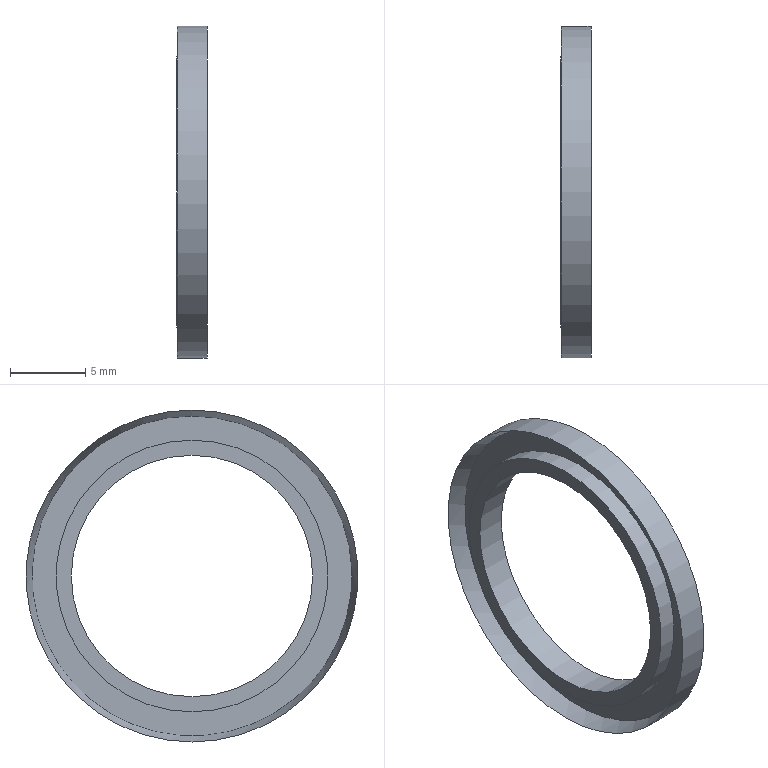Part | NX | features DATUM_CSYS 3, SKETCH 2, SWP104 1 | 1 solid | 7 faces | box 2 x 22 x 22 mm | volume 223.441 mm3 | plane 3 | cylinder 3 | cone 1 | commonest cylinder face diameters 16 x1 18 x1 22 x1
STEP:
#1=CARTESIAN_POINT('',(-0.4022,0.,9.));
#2=VERTEX_POINT('',#1);
#3=CARTESIAN_POINT('',(-0.4022,0.,0.));
#4=DIRECTION('',(-1.,0.,0.));
#5=DIRECTION('',(0.,0.,1.));
#6=AXIS2_PLACEMENT_3D('',#3,#4,#5);
#7=CIRCLE('',#6,9.);
#8=EDGE_CURVE('',#2,#2,#7,.T.);
#9=ORIENTED_EDGE('',*,*,#8,.F.);
#10=EDGE_LOOP('',(#9));
#11=FACE_BOUND('',#10,.T.);
#12=CARTESIAN_POINT('',(-0.4022,0.,10.6));
#13=VERTEX_POINT('',#12);
#14=CARTESIAN_POINT('',(-0.4022,0.,0.));
#15=DIRECTION('',(-1.,0.,0.));
#16=DIRECTION('',(0.,0.,1.));
#17=AXIS2_PLACEMENT_3D('',#14,#15,#16);
#18=CIRCLE('',#17,10.6);
#19=EDGE_CURVE('',#13,#13,#18,.T.);
#20=ORIENTED_EDGE('',*,*,#19,.T.);
#21=EDGE_LOOP('',(#20));
#22=FACE_BOUND('',#21,.T.);
#23=CARTESIAN_POINT('',(-0.4022,10.6,0.));
#24=DIRECTION('',(1.,0.,0.));
#25=DIRECTION('',(0.,0.,-1.));
#26=AXIS2_PLACEMENT_3D('',#23,#24,#25);
#27=PLANE('',#26);
#28=ADVANCED_FACE('',(#11,#22),#27,.F.);
#29=CARTESIAN_POINT('',(-1.602,0.,9.));
#30=VERTEX_POINT('',#29);
#31=CARTESIAN_POINT('',(-1.602,0.,0.));
#32=DIRECTION('',(-1.,0.,0.));
#33=DIRECTION('',(0.,0.,1.));
#34=AXIS2_PLACEMENT_3D('',#31,#32,#33);
#35=CIRCLE('',#34,9.);
#36=EDGE_CURVE('',#30,#30,#35,.T.);
#37=ORIENTED_EDGE('',*,*,#36,.F.);
#38=EDGE_LOOP('',(#37));
#39=FACE_BOUND('',#38,.T.);
#40=ORIENTED_EDGE('',*,*,#8,.T.);
#41=EDGE_LOOP('',(#40));
#42=FACE_BOUND('',#41,.T.);
#43=CARTESIAN_POINT('',(0.,0.,0.));
#44=DIRECTION('',(-1.,0.,0.));
#45=DIRECTION('',(0.,0.,1.));
#46=AXIS2_PLACEMENT_3D('',#43,#44,#45);
#47=CYLINDRICAL_SURFACE('',#46,9.);
#48=ADVANCED_FACE('',(#39,#42),#47,.T.);
#49=CARTESIAN_POINT('',(-1.602,0.,8.));
#50=VERTEX_POINT('',#49);
#51=CARTESIAN_POINT('',(-1.602,0.,0.));
#52=DIRECTION('',(-1.,0.,0.));
#53=DIRECTION('',(0.,0.,1.));
#54=AXIS2_PLACEMENT_3D('',#51,#52,#53);
#55=CIRCLE('',#54,8.);
#56=EDGE_CURVE('',#50,#50,#55,.T.);
#57=ORIENTED_EDGE('',*,*,#56,.F.);
#58=EDGE_LOOP('',(#57));
#59=FACE_BOUND('',#58,.T.);
#60=ORIENTED_EDGE('',*,*,#36,.T.);
#61=EDGE_LOOP('',(#60));
#62=FACE_BOUND('',#61,.T.);
#63=CARTESIAN_POINT('',(-1.602,9.,0.));
#64=DIRECTION('',(1.,0.,0.));
#65=DIRECTION('',(0.,0.,-1.));
#66=AXIS2_PLACEMENT_3D('',#63,#64,#65);
#67=PLANE('',#66);
#68=ADVANCED_FACE('',(#59,#62),#67,.F.);
#69=CARTESIAN_POINT('',(0.3978,0.,8.));
#70=VERTEX_POINT('',#69);
#71=CARTESIAN_POINT('',(0.3978,0.,0.));
#72=DIRECTION('',(-1.,0.,0.));
#73=DIRECTION('',(0.,0.,1.));
#74=AXIS2_PLACEMENT_3D('',#71,#72,#73);
#75=CIRCLE('',#74,8.);
#76=EDGE_CURVE('',#70,#70,#75,.T.);
#77=ORIENTED_EDGE('',*,*,#76,.F.);
#78=EDGE_LOOP('',(#77));
#79=FACE_BOUND('',#78,.T.);
#80=ORIENTED_EDGE('',*,*,#56,.T.);
#81=EDGE_LOOP('',(#80));
#82=FACE_BOUND('',#81,.T.);
#83=CARTESIAN_POINT('',(0.,0.,0.));
#84=DIRECTION('',(-1.,0.,0.));
#85=DIRECTION('',(0.,0.,1.));
#86=AXIS2_PLACEMENT_3D('',#83,#84,#85);
#87=CYLINDRICAL_SURFACE('',#86,8.);
#88=ADVANCED_FACE('',(#79,#82),#87,.F.);
#89=CARTESIAN_POINT('',(0.3978,0.,11.));
#90=VERTEX_POINT('',#89);
#91=CARTESIAN_POINT('',(0.3978,0.,0.));
#92=DIRECTION('',(-1.,0.,0.));
#93=DIRECTION('',(0.,0.,1.));
#94=AXIS2_PLACEMENT_3D('',#91,#92,#93);
#95=CIRCLE('',#94,11.);
#96=EDGE_CURVE('',#90,#90,#95,.T.);
#97=ORIENTED_EDGE('',*,*,#96,.F.);
#98=EDGE_LOOP('',(#97));
#99=FACE_BOUND('',#98,.T.);
#100=ORIENTED_EDGE('',*,*,#76,.T.);
#101=EDGE_LOOP('',(#100));
#102=FACE_BOUND('',#101,.T.);
#103=CARTESIAN_POINT('',(0.3978,8.,0.));
#104=DIRECTION('',(-1.,0.,0.));
#105=DIRECTION('',(0.,0.,1.));
#106=AXIS2_PLACEMENT_3D('',#103,#104,#105);
#107=PLANE('',#106);
#108=ADVANCED_FACE('',(#99,#102),#107,.F.);
#109=CARTESIAN_POINT('',(-1.581,0.,11.));
#110=VERTEX_POINT('',#109);
#111=CARTESIAN_POINT('',(-1.581,0.,0.));
#112=DIRECTION('',(-1.,0.,0.));
#113=DIRECTION('',(0.,0.,1.));
#114=AXIS2_PLACEMENT_3D('',#111,#112,#113);
#115=CIRCLE('',#114,11.);
#116=EDGE_CURVE('',#110,#110,#115,.T.);
#117=ORIENTED_EDGE('',*,*,#116,.F.);
#118=EDGE_LOOP('',(#117));
#119=FACE_BOUND('',#118,.T.);
#120=ORIENTED_EDGE('',*,*,#96,.T.);
#121=EDGE_LOOP('',(#120));
#122=FACE_BOUND('',#121,.T.);
#123=CARTESIAN_POINT('',(0.,0.,0.));
#124=DIRECTION('',(-1.,0.,0.));
#125=DIRECTION('',(0.,0.,1.));
#126=AXIS2_PLACEMENT_3D('',#123,#124,#125);
#127=CYLINDRICAL_SURFACE('',#126,11.);
#128=ADVANCED_FACE('',(#119,#122),#127,.T.);
#129=ORIENTED_EDGE('',*,*,#19,.F.);
#130=EDGE_LOOP('',(#129));
#131=FACE_BOUND('',#130,.T.);
#132=ORIENTED_EDGE('',*,*,#116,.T.);
#133=EDGE_LOOP('',(#132));
#134=FACE_BOUND('',#133,.T.);
#135=CARTESIAN_POINT('',(-1.581,0.,0.));
#136=DIRECTION('',(-1.,0.,0.));
#137=DIRECTION('',(0.,0.,1.));
#138=AXIS2_PLACEMENT_3D('',#135,#136,#137);
#139=CONICAL_SURFACE('',#138,11.,0.3272);
#140=ADVANCED_FACE('',(#131,#134),#139,.F.);
#141=CLOSED_SHELL('',(#28,#48,#68,#88,#108,#128,#140));
#142=MANIFOLD_SOLID_BREP('',#141);
#143=(LENGTH_UNIT()NAMED_UNIT(*)SI_UNIT(.MILLI.,.METRE.));
#144=UNCERTAINTY_MEASURE_WITH_UNIT(LENGTH_MEASURE(0.00001),#143,'','');
#145=(NAMED_UNIT(*)PLANE_ANGLE_UNIT()SI_UNIT($,.RADIAN.));
#146=(NAMED_UNIT(*)SI_UNIT($,.STERADIAN.)SOLID_ANGLE_UNIT());
#147=(GEOMETRIC_REPRESENTATION_CONTEXT(3)GLOBAL_UNCERTAINTY_ASSIGNED_CONTEXT((#144))GLOBAL_UNIT_ASSIGNED_CONTEXT((#143,#145,#146))REPRESENTATION_CONTEXT('',''));
#148=ADVANCED_BREP_SHAPE_REPRESENTATION('',(#142),#147);